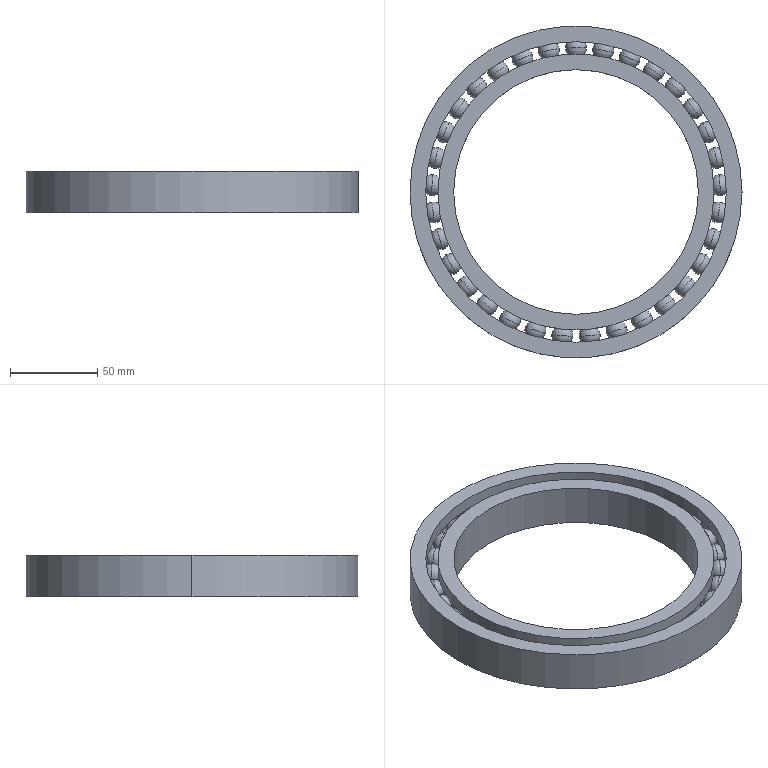Part | NX | features BREP 35 | 35 solids | 154 faces | box 190 x 190 x 24 mm | volume 228051 mm3 | sphere 132 | cylinder 10 | torus 6 | plane 4 | cone 2 | commonest cylinder face diameters 158 x4 140 x2 172 x2 190 x2